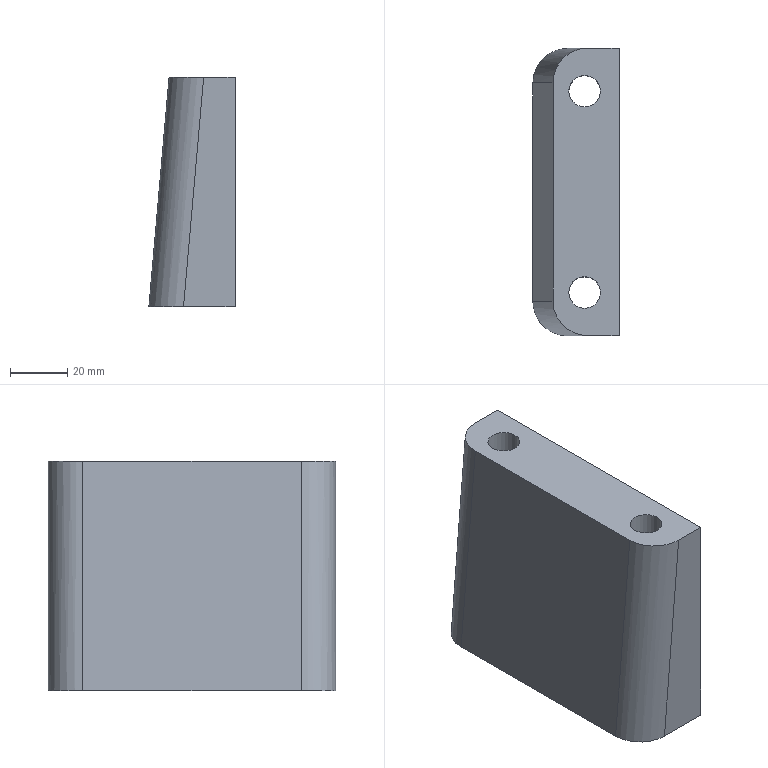Part | STEP file | solid 8 | 1 solid | 18 faces | box 30 x 100 x 80 mm | volume 186268 mm3 | plane 8 | cylinder 8 | cone 2 | commonest cylinder face diameters 11 x2 18 x2 24 x2 9 x1 10 x1